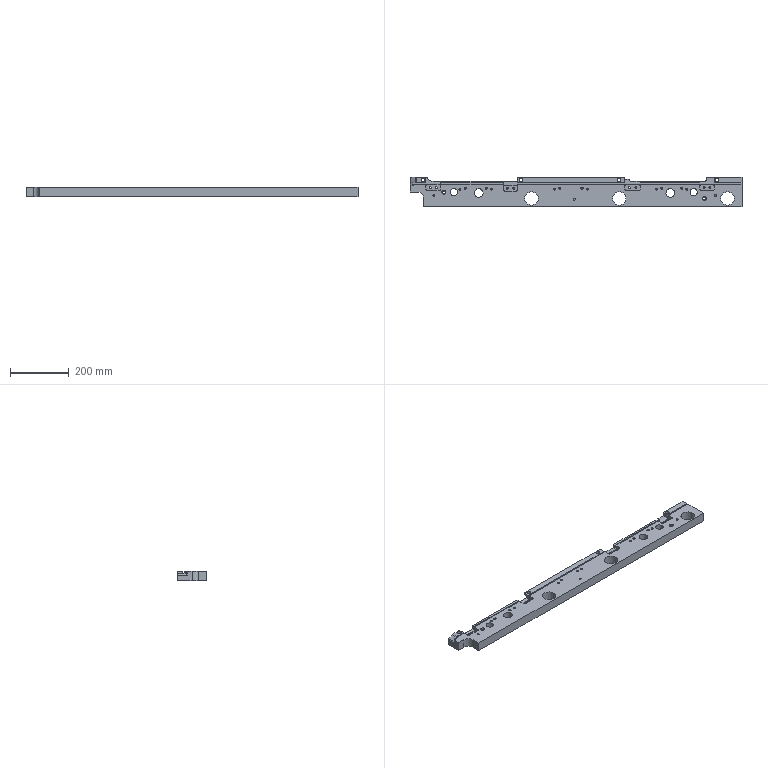Part | STEP file | gslz 2016.10.28-13_id318_x_t | 1 solid | 167 faces | box 1135 x 100 x 32 mm | volume 2853075 mm3 | cylinder 80 | plane 68 | cone 19 | commonest cylinder face diameters 10 x24 6.8 x21 6 x7 8 x6 5.2 x4 13 x4